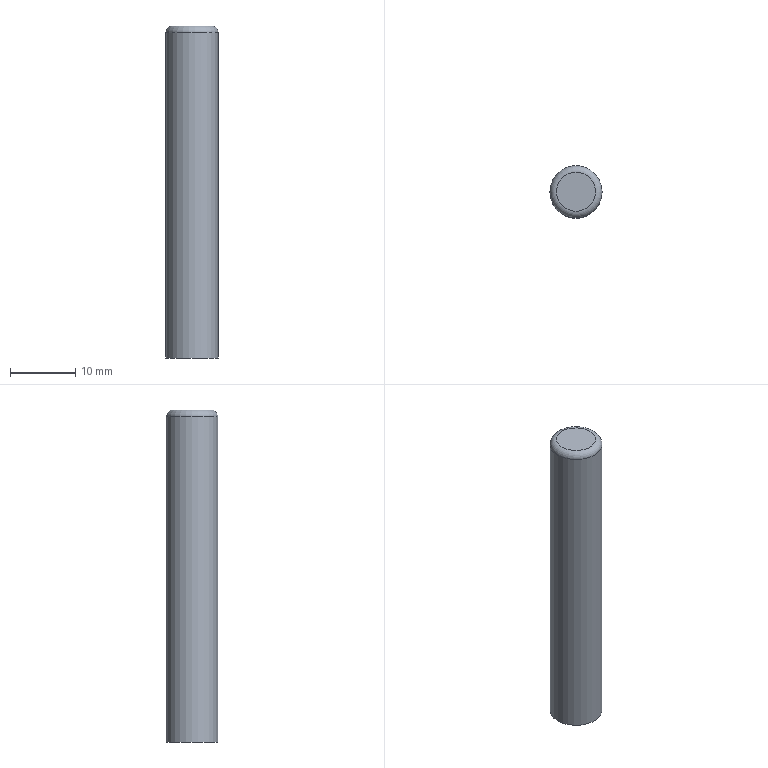Part | STEP file | lll_id3782_x_t | 1 solid | 4 faces | box 8 x 8 x 51 mm | volume 2558 mm3 | plane 2 | cylinder 1 | torus 1 | commonest cylinder face diameters 8 x1
STEP:
#1=CARTESIAN_POINT('',(4019.,-535.677,118.75));
#2=VERTEX_POINT('',#1);
#3=CARTESIAN_POINT('',(4023.,-535.677,118.75));
#4=DIRECTION('',(0.,0.,-1.));
#5=DIRECTION('',(-1.,0.,0.));
#6=AXIS2_PLACEMENT_3D('',#3,#4,#5);
#7=CIRCLE('',#6,4.);
#8=EDGE_CURVE('',#2,#2,#7,.T.);
#9=ORIENTED_EDGE('',*,*,#8,.F.);
#10=EDGE_LOOP('',(#9));
#11=FACE_BOUND('',#10,.T.);
#12=CARTESIAN_POINT('',(4027.,-535.677,168.75));
#13=VERTEX_POINT('',#12);
#14=CARTESIAN_POINT('',(4023.,-535.677,168.75));
#15=DIRECTION('',(0.,0.,-1.));
#16=DIRECTION('',(1.,0.,0.));
#17=AXIS2_PLACEMENT_3D('',#14,#15,#16);
#18=CIRCLE('',#17,4.);
#19=EDGE_CURVE('',#13,#13,#18,.T.);
#20=ORIENTED_EDGE('',*,*,#19,.T.);
#21=EDGE_LOOP('',(#20));
#22=FACE_BOUND('',#21,.T.);
#23=CARTESIAN_POINT('',(4023.,-535.677,169.75));
#24=DIRECTION('',(0.,0.,-1.));
#25=DIRECTION('',(-1.,0.,0.));
#26=AXIS2_PLACEMENT_3D('',#23,#24,#25);
#27=CYLINDRICAL_SURFACE('',#26,4.);
#28=ADVANCED_FACE('',(#11,#22),#27,.T.);
#29=ORIENTED_EDGE('',*,*,#19,.F.);
#30=EDGE_LOOP('',(#29));
#31=FACE_BOUND('',#30,.T.);
#32=CARTESIAN_POINT('',(4026.,-535.677,169.75));
#33=VERTEX_POINT('',#32);
#34=CARTESIAN_POINT('',(4023.,-535.677,169.75));
#35=DIRECTION('',(0.,0.,1.));
#36=DIRECTION('',(1.,0.,0.));
#37=AXIS2_PLACEMENT_3D('',#34,#35,#36);
#38=CIRCLE('',#37,3.);
#39=EDGE_CURVE('',#33,#33,#38,.T.);
#40=ORIENTED_EDGE('',*,*,#39,.F.);
#41=EDGE_LOOP('',(#40));
#42=FACE_BOUND('',#41,.T.);
#43=CARTESIAN_POINT('',(4023.,-535.677,168.75));
#44=DIRECTION('',(0.,0.,1.));
#45=DIRECTION('',(1.,0.,0.));
#46=AXIS2_PLACEMENT_3D('',#43,#44,#45);
#47=TOROIDAL_SURFACE('',#46,3.,1.);
#48=ADVANCED_FACE('',(#31,#42),#47,.T.);
#49=ORIENTED_EDGE('',*,*,#8,.T.);
#50=EDGE_LOOP('',(#49));
#51=FACE_OUTER_BOUND('',#50,.T.);
#52=CARTESIAN_POINT('',(4021.4,-524.378,118.75));
#53=DIRECTION('',(0.,0.,-1.));
#54=DIRECTION('',(-1.,0.,0.));
#55=AXIS2_PLACEMENT_3D('',#52,#53,#54);
#56=PLANE('',#55);
#57=ADVANCED_FACE('',(#51),#56,.T.);
#58=ORIENTED_EDGE('',*,*,#39,.T.);
#59=EDGE_LOOP('',(#58));
#60=FACE_OUTER_BOUND('',#59,.T.);
#61=CARTESIAN_POINT('',(4023.,-538.135,169.75));
#62=DIRECTION('',(0.,0.,1.));
#63=DIRECTION('',(1.,0.,0.));
#64=AXIS2_PLACEMENT_3D('',#61,#62,#63);
#65=PLANE('',#64);
#66=ADVANCED_FACE('',(#60),#65,.T.);
#67=CLOSED_SHELL('',(#28,#48,#57,#66));
#68=MANIFOLD_SOLID_BREP('',#67);
#69=(LENGTH_UNIT()NAMED_UNIT(*)SI_UNIT(.MILLI.,.METRE.));
#70=UNCERTAINTY_MEASURE_WITH_UNIT(LENGTH_MEASURE(0.00002),#69,'','');
#71=(NAMED_UNIT(*)PLANE_ANGLE_UNIT()SI_UNIT($,.RADIAN.));
#72=PLANE_ANGLE_MEASURE_WITH_UNIT(PLANE_ANGLE_MEASURE(0.01745),#71);
#73=DIMENSIONAL_EXPONENTS(0.,0.,0.,0.,0.,0.,0.);
#74=(CONVERSION_BASED_UNIT('DEGREE',#72)NAMED_UNIT(#73)PLANE_ANGLE_UNIT());
#75=(NAMED_UNIT(*)SI_UNIT($,.STERADIAN.)SOLID_ANGLE_UNIT());
#76=(GEOMETRIC_REPRESENTATION_CONTEXT(3)GLOBAL_UNCERTAINTY_ASSIGNED_CONTEXT((#70))GLOBAL_UNIT_ASSIGNED_CONTEXT((#69,#74,#75))REPRESENTATION_CONTEXT('',''));
#77=ADVANCED_BREP_SHAPE_REPRESENTATION('',(#68),#76);